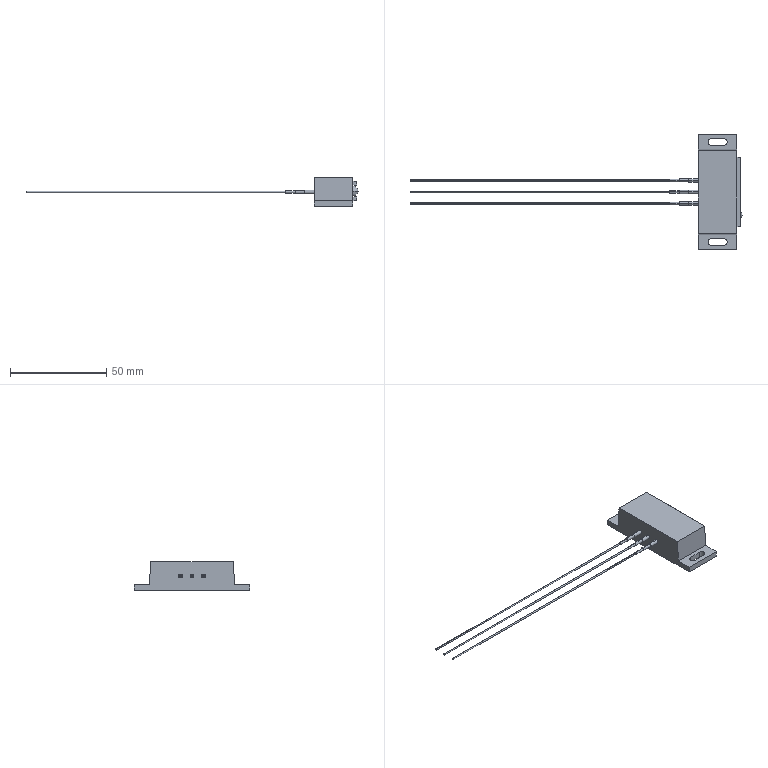Part | SolidWorks | features BaseBody 1 | 1 solid | 68 faces | box 172.7 x 60 x 15 mm | volume 14511 mm3 | plane 36 | cylinder 30 | spline 2 | commonest cylinder face diameters 0.8 x6 1.2 x6 1.6 x6 2 x6 3.4 x6